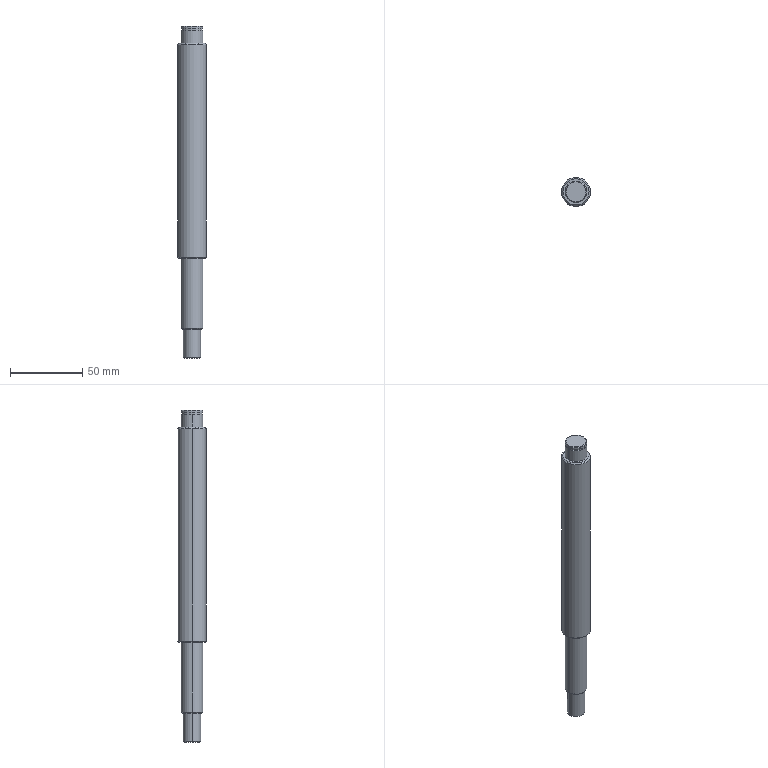Part | SolidWorks | features BaseBody 1 | 1 solid | 29 faces | box 20 x 20 x 230 mm | volume 59762 mm3 | cylinder 12 | cone 10 | plane 7 | commonest cylinder face diameters 15 x6 12 x2 14.3 x2 20 x2
STEP:
#1=CARTESIAN_POINT('',(-5.5,0.,-230.));
#2=VERTEX_POINT('',#1);
#3=CARTESIAN_POINT('',(5.5,0.,-230.));
#4=VERTEX_POINT('',#3);
#5=CARTESIAN_POINT('',(0.,0.,-230.));
#6=DIRECTION('',(0.,0.,-1.));
#7=DIRECTION('',(-1.,0.,0.));
#8=AXIS2_PLACEMENT_3D('',#5,#6,#7);
#9=CIRCLE('',#8,5.5);
#10=EDGE_CURVE('',#2,#4,#9,.T.);
#11=ORIENTED_EDGE('',*,*,#10,.F.);
#12=CARTESIAN_POINT('',(-6.,0.,-229.5));
#13=VERTEX_POINT('',#12);
#14=CARTESIAN_POINT('',(-6.,0.,-229.5));
#15=DIRECTION('',(-0.7071,0.,0.7071));
#16=VECTOR('',#15,1000.);
#17=LINE('',#14,#16);
#18=EDGE_CURVE('',#2,#13,#17,.T.);
#19=ORIENTED_EDGE('',*,*,#18,.T.);
#20=CARTESIAN_POINT('',(6.,0.,-229.5));
#21=VERTEX_POINT('',#20);
#22=CARTESIAN_POINT('',(0.,0.,-229.5));
#23=DIRECTION('',(0.,0.,-1.));
#24=DIRECTION('',(-1.,0.,0.));
#25=AXIS2_PLACEMENT_3D('',#22,#23,#24);
#26=CIRCLE('',#25,6.);
#27=EDGE_CURVE('',#13,#21,#26,.T.);
#28=ORIENTED_EDGE('',*,*,#27,.T.);
#29=CARTESIAN_POINT('',(6.,0.,-229.5));
#30=DIRECTION('',(0.7071,0.,0.7071));
#31=VECTOR('',#30,1000.);
#32=LINE('',#29,#31);
#33=EDGE_CURVE('',#4,#21,#32,.T.);
#34=ORIENTED_EDGE('',*,*,#33,.F.);
#35=EDGE_LOOP('',(#11,#19,#28,#34));
#36=FACE_OUTER_BOUND('',#35,.T.);
#37=CARTESIAN_POINT('',(0.,0.,-229.5));
#38=DIRECTION('',(0.,0.,1.));
#39=DIRECTION('',(1.,0.,0.));
#40=AXIS2_PLACEMENT_3D('',#37,#38,#39);
#41=CONICAL_SURFACE('',#40,6.,0.7854);
#42=ADVANCED_FACE('',(#36),#41,.T.);
#43=CARTESIAN_POINT('',(-6.,0.,-210.));
#44=VERTEX_POINT('',#43);
#45=CARTESIAN_POINT('',(6.,0.,-210.));
#46=VERTEX_POINT('',#45);
#47=CARTESIAN_POINT('',(0.,0.,-210.));
#48=DIRECTION('',(0.,0.,-1.));
#49=DIRECTION('',(-1.,0.,0.));
#50=AXIS2_PLACEMENT_3D('',#47,#48,#49);
#51=CIRCLE('',#50,6.);
#52=EDGE_CURVE('',#44,#46,#51,.T.);
#53=ORIENTED_EDGE('',*,*,#52,.T.);
#54=CARTESIAN_POINT('',(6.,0.,-230.));
#55=DIRECTION('',(0.,0.,-1.));
#56=VECTOR('',#55,1000.);
#57=LINE('',#54,#56);
#58=EDGE_CURVE('',#46,#21,#57,.T.);
#59=ORIENTED_EDGE('',*,*,#58,.T.);
#60=ORIENTED_EDGE('',*,*,#27,.F.);
#61=CARTESIAN_POINT('',(-6.,0.,-230.));
#62=DIRECTION('',(0.,0.,-1.));
#63=VECTOR('',#62,1000.);
#64=LINE('',#61,#63);
#65=EDGE_CURVE('',#44,#13,#64,.T.);
#66=ORIENTED_EDGE('',*,*,#65,.F.);
#67=EDGE_LOOP('',(#53,#59,#60,#66));
#68=FACE_OUTER_BOUND('',#67,.T.);
#69=CARTESIAN_POINT('',(0.,0.,-230.));
#70=DIRECTION('',(0.,0.,-1.));
#71=DIRECTION('',(-1.,0.,0.));
#72=AXIS2_PLACEMENT_3D('',#69,#70,#71);
#73=CYLINDRICAL_SURFACE('',#72,6.);
#74=ADVANCED_FACE('',(#68),#73,.T.);
#75=CARTESIAN_POINT('',(-6.886,0.,-210.));
#76=VERTEX_POINT('',#75);
#77=CARTESIAN_POINT('',(6.886,0.,-210.));
#78=VERTEX_POINT('',#77);
#79=CARTESIAN_POINT('',(0.,0.,-210.));
#80=DIRECTION('',(0.,0.,-1.));
#81=DIRECTION('',(-1.,0.,0.));
#82=AXIS2_PLACEMENT_3D('',#79,#80,#81);
#83=CIRCLE('',#82,6.886);
#84=EDGE_CURVE('',#76,#78,#83,.T.);
#85=ORIENTED_EDGE('',*,*,#84,.F.);
#86=CARTESIAN_POINT('',(-7.5,0.,-209.387));
#87=VERTEX_POINT('',#86);
#88=CARTESIAN_POINT('',(-7.5,0.,-209.387));
#89=DIRECTION('',(-0.7071,0.,0.7071));
#90=VECTOR('',#89,1000.);
#91=LINE('',#88,#90);
#92=EDGE_CURVE('',#76,#87,#91,.T.);
#93=ORIENTED_EDGE('',*,*,#92,.T.);
#94=CARTESIAN_POINT('',(7.5,0.,-209.387));
#95=VERTEX_POINT('',#94);
#96=CARTESIAN_POINT('',(0.,0.,-209.387));
#97=DIRECTION('',(0.,0.,-1.));
#98=DIRECTION('',(-1.,0.,0.));
#99=AXIS2_PLACEMENT_3D('',#96,#97,#98);
#100=CIRCLE('',#99,7.5);
#101=EDGE_CURVE('',#87,#95,#100,.T.);
#102=ORIENTED_EDGE('',*,*,#101,.T.);
#103=CARTESIAN_POINT('',(7.5,0.,-209.387));
#104=DIRECTION('',(0.7071,0.,0.7071));
#105=VECTOR('',#104,1000.);
#106=LINE('',#103,#105);
#107=EDGE_CURVE('',#78,#95,#106,.T.);
#108=ORIENTED_EDGE('',*,*,#107,.F.);
#109=EDGE_LOOP('',(#85,#93,#102,#108));
#110=FACE_OUTER_BOUND('',#109,.T.);
#111=CARTESIAN_POINT('',(0.,0.,-209.387));
#112=DIRECTION('',(0.,0.,1.));
#113=DIRECTION('',(1.,0.,0.));
#114=AXIS2_PLACEMENT_3D('',#111,#112,#113);
#115=CONICAL_SURFACE('',#114,7.5,0.7854);
#116=ADVANCED_FACE('',(#110),#115,.T.);
#117=CARTESIAN_POINT('',(-7.5,0.,-161.));
#118=VERTEX_POINT('',#117);
#119=CARTESIAN_POINT('',(7.5,0.,-161.));
#120=VERTEX_POINT('',#119);
#121=CARTESIAN_POINT('',(0.,0.,-161.));
#122=DIRECTION('',(0.,0.,-1.));
#123=DIRECTION('',(-1.,0.,0.));
#124=AXIS2_PLACEMENT_3D('',#121,#122,#123);
#125=CIRCLE('',#124,7.5);
#126=EDGE_CURVE('',#118,#120,#125,.T.);
#127=ORIENTED_EDGE('',*,*,#126,.T.);
#128=CARTESIAN_POINT('',(7.5,0.,-230.));
#129=DIRECTION('',(0.,0.,-1.));
#130=VECTOR('',#129,1000.);
#131=LINE('',#128,#130);
#132=EDGE_CURVE('',#120,#95,#131,.T.);
#133=ORIENTED_EDGE('',*,*,#132,.T.);
#134=ORIENTED_EDGE('',*,*,#101,.F.);
#135=CARTESIAN_POINT('',(-7.5,0.,-230.));
#136=DIRECTION('',(0.,0.,-1.));
#137=VECTOR('',#136,1000.);
#138=LINE('',#135,#137);
#139=EDGE_CURVE('',#118,#87,#138,.T.);
#140=ORIENTED_EDGE('',*,*,#139,.F.);
#141=EDGE_LOOP('',(#127,#133,#134,#140));
#142=FACE_OUTER_BOUND('',#141,.T.);
#143=CARTESIAN_POINT('',(0.,0.,-230.));
#144=DIRECTION('',(0.,0.,-1.));
#145=DIRECTION('',(-1.,0.,0.));
#146=AXIS2_PLACEMENT_3D('',#143,#144,#145);
#147=CYLINDRICAL_SURFACE('',#146,7.5);
#148=ADVANCED_FACE('',(#142),#147,.T.);
#149=CARTESIAN_POINT('',(-9.08,0.,-161.));
#150=VERTEX_POINT('',#149);
#151=CARTESIAN_POINT('',(9.08,0.,-161.));
#152=VERTEX_POINT('',#151);
#153=CARTESIAN_POINT('',(0.,0.,-161.));
#154=DIRECTION('',(0.,0.,-1.));
#155=DIRECTION('',(-1.,0.,0.));
#156=AXIS2_PLACEMENT_3D('',#153,#154,#155);
#157=CIRCLE('',#156,9.08);
#158=EDGE_CURVE('',#150,#152,#157,.T.);
#159=ORIENTED_EDGE('',*,*,#158,.F.);
#160=CARTESIAN_POINT('',(-10.,0.,-160.08));
#161=VERTEX_POINT('',#160);
#162=CARTESIAN_POINT('',(-10.,0.,-160.08));
#163=DIRECTION('',(-0.7071,0.,0.7071));
#164=VECTOR('',#163,1000.);
#165=LINE('',#162,#164);
#166=EDGE_CURVE('',#150,#161,#165,.T.);
#167=ORIENTED_EDGE('',*,*,#166,.T.);
#168=CARTESIAN_POINT('',(10.,0.,-160.08));
#169=VERTEX_POINT('',#168);
#170=CARTESIAN_POINT('',(0.,0.,-160.08));
#171=DIRECTION('',(0.,0.,-1.));
#172=DIRECTION('',(-1.,0.,0.));
#173=AXIS2_PLACEMENT_3D('',#170,#171,#172);
#174=CIRCLE('',#173,10.);
#175=EDGE_CURVE('',#161,#169,#174,.T.);
#176=ORIENTED_EDGE('',*,*,#175,.T.);
#177=CARTESIAN_POINT('',(10.,0.,-160.08));
#178=DIRECTION('',(0.7071,0.,0.7071));
#179=VECTOR('',#178,1000.);
#180=LINE('',#177,#179);
#181=EDGE_CURVE('',#152,#169,#180,.T.);
#182=ORIENTED_EDGE('',*,*,#181,.F.);
#183=EDGE_LOOP('',(#159,#167,#176,#182));
#184=FACE_OUTER_BOUND('',#183,.T.);
#185=CARTESIAN_POINT('',(0.,0.,-160.08));
#186=DIRECTION('',(0.,0.,1.));
#187=DIRECTION('',(1.,0.,0.));
#188=AXIS2_PLACEMENT_3D('',#185,#186,#187);
#189=CONICAL_SURFACE('',#188,10.,0.7854);
#190=ADVANCED_FACE('',(#184),#189,.T.);
#191=CARTESIAN_POINT('',(-10.,0.,-12.92));
#192=VERTEX_POINT('',#191);
#193=CARTESIAN_POINT('',(10.,0.,-12.92));
#194=VERTEX_POINT('',#193);
#195=CARTESIAN_POINT('',(0.,0.,-12.92));
#196=DIRECTION('',(0.,0.,-1.));
#197=DIRECTION('',(-1.,0.,0.));
#198=AXIS2_PLACEMENT_3D('',#195,#196,#197);
#199=CIRCLE('',#198,10.);
#200=EDGE_CURVE('',#192,#194,#199,.T.);
#201=ORIENTED_EDGE('',*,*,#200,.T.);
#202=CARTESIAN_POINT('',(10.,0.,-230.));
#203=DIRECTION('',(0.,0.,-1.));
#204=VECTOR('',#203,1000.);
#205=LINE('',#202,#204);
#206=EDGE_CURVE('',#194,#169,#205,.T.);
#207=ORIENTED_EDGE('',*,*,#206,.T.);
#208=ORIENTED_EDGE('',*,*,#175,.F.);
#209=CARTESIAN_POINT('',(-10.,0.,-230.));
#210=DIRECTION('',(0.,0.,-1.));
#211=VECTOR('',#210,1000.);
#212=LINE('',#209,#211);
#213=EDGE_CURVE('',#192,#161,#212,.T.);
#214=ORIENTED_EDGE('',*,*,#213,.F.);
#215=EDGE_LOOP('',(#201,#207,#208,#214));
#216=FACE_OUTER_BOUND('',#215,.T.);
#217=CARTESIAN_POINT('',(0.,0.,-230.));
#218=DIRECTION('',(0.,0.,-1.));
#219=DIRECTION('',(-1.,0.,0.));
#220=AXIS2_PLACEMENT_3D('',#217,#218,#219);
#221=CYLINDRICAL_SURFACE('',#220,10.);
#222=ADVANCED_FACE('',(#216),#221,.T.);
#223=CARTESIAN_POINT('',(-9.08,0.,-12.));
#224=VERTEX_POINT('',#223);
#225=CARTESIAN_POINT('',(9.08,0.,-12.));
#226=VERTEX_POINT('',#225);
#227=CARTESIAN_POINT('',(0.,0.,-12.));
#228=DIRECTION('',(0.,0.,-1.));
#229=DIRECTION('',(-1.,0.,0.));
#230=AXIS2_PLACEMENT_3D('',#227,#228,#229);
#231=CIRCLE('',#230,9.08);
#232=EDGE_CURVE('',#224,#226,#231,.T.);
#233=ORIENTED_EDGE('',*,*,#232,.T.);
#234=CARTESIAN_POINT('',(9.08,0.,-12.));
#235=DIRECTION('',(0.7071,0.,-0.7071));
#236=VECTOR('',#235,1000.);
#237=LINE('',#234,#236);
#238=EDGE_CURVE('',#226,#194,#237,.T.);
#239=ORIENTED_EDGE('',*,*,#238,.T.);
#240=ORIENTED_EDGE('',*,*,#200,.F.);
#241=CARTESIAN_POINT('',(-9.08,0.,-12.));
#242=DIRECTION('',(-0.7071,0.,-0.7071));
#243=VECTOR('',#242,1000.);
#244=LINE('',#241,#243);
#245=EDGE_CURVE('',#224,#192,#244,.T.);
#246=ORIENTED_EDGE('',*,*,#245,.F.);
#247=EDGE_LOOP('',(#233,#239,#240,#246));
#248=FACE_OUTER_BOUND('',#247,.T.);
#249=CARTESIAN_POINT('',(0.,0.,-12.));
#250=DIRECTION('',(0.,0.,-1.));
#251=DIRECTION('',(-1.,0.,0.));
#252=AXIS2_PLACEMENT_3D('',#249,#250,#251);
#253=CONICAL_SURFACE('',#252,9.08,0.7854);
#254=ADVANCED_FACE('',(#248),#253,.T.);
#255=CARTESIAN_POINT('',(-7.5,0.,-3.));
#256=VERTEX_POINT('',#255);
#257=CARTESIAN_POINT('',(7.5,0.,-3.));
#258=VERTEX_POINT('',#257);
#259=CARTESIAN_POINT('',(0.,0.,-3.));
#260=DIRECTION('',(0.,0.,-1.));
#261=DIRECTION('',(-1.,0.,0.));
#262=AXIS2_PLACEMENT_3D('',#259,#260,#261);
#263=CIRCLE('',#262,7.5);
#264=EDGE_CURVE('',#256,#258,#263,.T.);
#265=ORIENTED_EDGE('',*,*,#264,.T.);
#266=CARTESIAN_POINT('',(7.5,0.,-12.));
#267=VERTEX_POINT('',#266);
#268=CARTESIAN_POINT('',(7.5,0.,-230.));
#269=DIRECTION('',(0.,0.,-1.));
#270=VECTOR('',#269,1000.);
#271=LINE('',#268,#270);
#272=EDGE_CURVE('',#258,#267,#271,.T.);
#273=ORIENTED_EDGE('',*,*,#272,.T.);
#274=CARTESIAN_POINT('',(-7.5,0.,-12.));
#275=VERTEX_POINT('',#274);
#276=CARTESIAN_POINT('',(0.,0.,-12.));
#277=DIRECTION('',(0.,0.,-1.));
#278=DIRECTION('',(-1.,0.,0.));
#279=AXIS2_PLACEMENT_3D('',#276,#277,#278);
#280=CIRCLE('',#279,7.5);
#281=EDGE_CURVE('',#275,#267,#280,.T.);
#282=ORIENTED_EDGE('',*,*,#281,.F.);
#283=CARTESIAN_POINT('',(-7.5,0.,-230.));
#284=DIRECTION('',(0.,0.,-1.));
#285=VECTOR('',#284,1000.);
#286=LINE('',#283,#285);
#287=EDGE_CURVE('',#256,#275,#286,.T.);
#288=ORIENTED_EDGE('',*,*,#287,.F.);
#289=EDGE_LOOP('',(#265,#273,#282,#288));
#290=FACE_OUTER_BOUND('',#289,.T.);
#291=CARTESIAN_POINT('',(0.,0.,-230.));
#292=DIRECTION('',(0.,0.,-1.));
#293=DIRECTION('',(-1.,0.,0.));
#294=AXIS2_PLACEMENT_3D('',#291,#292,#293);
#295=CYLINDRICAL_SURFACE('',#294,7.5);
#296=ADVANCED_FACE('',(#290),#295,.T.);
#297=CARTESIAN_POINT('',(-7.15,0.,-1.85));
#298=VERTEX_POINT('',#297);
#299=CARTESIAN_POINT('',(7.15,0.,-1.85));
#300=VERTEX_POINT('',#299);
#301=CARTESIAN_POINT('',(0.,0.,-1.85));
#302=DIRECTION('',(0.,0.,-1.));
#303=DIRECTION('',(-1.,0.,0.));
#304=AXIS2_PLACEMENT_3D('',#301,#302,#303);
#305=CIRCLE('',#304,7.15);
#306=EDGE_CURVE('',#298,#300,#305,.T.);
#307=ORIENTED_EDGE('',*,*,#306,.T.);
#308=CARTESIAN_POINT('',(7.15,0.,-3.));
#309=VERTEX_POINT('',#308);
#310=CARTESIAN_POINT('',(7.15,0.,-230.));
#311=DIRECTION('',(0.,0.,-1.));
#312=VECTOR('',#311,1000.);
#313=LINE('',#310,#312);
#314=EDGE_CURVE('',#300,#309,#313,.T.);
#315=ORIENTED_EDGE('',*,*,#314,.T.);
#316=CARTESIAN_POINT('',(-7.15,0.,-3.));
#317=VERTEX_POINT('',#316);
#318=CARTESIAN_POINT('',(0.,0.,-3.));
#319=DIRECTION('',(0.,0.,-1.));
#320=DIRECTION('',(-1.,0.,0.));
#321=AXIS2_PLACEMENT_3D('',#318,#319,#320);
#322=CIRCLE('',#321,7.15);
#323=EDGE_CURVE('',#317,#309,#322,.T.);
#324=ORIENTED_EDGE('',*,*,#323,.F.);
#325=CARTESIAN_POINT('',(-7.15,0.,-230.));
#326=DIRECTION('',(0.,0.,-1.));
#327=VECTOR('',#326,1000.);
#328=LINE('',#325,#327);
#329=EDGE_CURVE('',#298,#317,#328,.T.);
#330=ORIENTED_EDGE('',*,*,#329,.F.);
#331=EDGE_LOOP('',(#307,#315,#324,#330));
#332=FACE_OUTER_BOUND('',#331,.T.);
#333=CARTESIAN_POINT('',(0.,0.,-230.));
#334=DIRECTION('',(0.,0.,-1.));
#335=DIRECTION('',(-1.,0.,0.));
#336=AXIS2_PLACEMENT_3D('',#333,#334,#335);
#337=CYLINDRICAL_SURFACE('',#336,7.15);
#338=ADVANCED_FACE('',(#332),#337,.T.);
#339=CARTESIAN_POINT('',(-7.5,0.,-0.5));
#340=VERTEX_POINT('',#339);
#341=CARTESIAN_POINT('',(7.5,0.,-0.5));
#342=VERTEX_POINT('',#341);
#343=CARTESIAN_POINT('',(0.,0.,-0.5));
#344=DIRECTION('',(0.,0.,-1.));
#345=DIRECTION('',(-1.,0.,0.));
#346=AXIS2_PLACEMENT_3D('',#343,#344,#345);
#347=CIRCLE('',#346,7.5);
#348=EDGE_CURVE('',#340,#342,#347,.T.);
#349=ORIENTED_EDGE('',*,*,#348,.T.);
#350=CARTESIAN_POINT('',(7.5,0.,-1.85));
#351=VERTEX_POINT('',#350);
#352=CARTESIAN_POINT('',(7.5,0.,-230.));
#353=DIRECTION('',(0.,0.,-1.));
#354=VECTOR('',#353,1000.);
#355=LINE('',#352,#354);
#356=EDGE_CURVE('',#342,#351,#355,.T.);
#357=ORIENTED_EDGE('',*,*,#356,.T.);
#358=CARTESIAN_POINT('',(-7.5,0.,-1.85));
#359=VERTEX_POINT('',#358);
#360=CARTESIAN_POINT('',(0.,0.,-1.85));
#361=DIRECTION('',(0.,0.,-1.));
#362=DIRECTION('',(-1.,0.,0.));
#363=AXIS2_PLACEMENT_3D('',#360,#361,#362);
#364=CIRCLE('',#363,7.5);
#365=EDGE_CURVE('',#359,#351,#364,.T.);
#366=ORIENTED_EDGE('',*,*,#365,.F.);
#367=CARTESIAN_POINT('',(-7.5,0.,-230.));
#368=DIRECTION('',(0.,0.,-1.));
#369=VECTOR('',#368,1000.);
#370=LINE('',#367,#369);
#371=EDGE_CURVE('',#340,#359,#370,.T.);
#372=ORIENTED_EDGE('',*,*,#371,.F.);
#373=EDGE_LOOP('',(#349,#357,#366,#372));
#374=FACE_OUTER_BOUND('',#373,.T.);
#375=CARTESIAN_POINT('',(0.,0.,-230.));
#376=DIRECTION('',(0.,0.,-1.));
#377=DIRECTION('',(-1.,0.,0.));
#378=AXIS2_PLACEMENT_3D('',#375,#376,#377);
#379=CYLINDRICAL_SURFACE('',#378,7.5);
#380=ADVANCED_FACE('',(#374),#379,.T.);
#381=CARTESIAN_POINT('',(-7.,0.,0.));
#382=VERTEX_POINT('',#381);
#383=CARTESIAN_POINT('',(7.,0.,0.));
#384=VERTEX_POINT('',#383);
#385=CARTESIAN_POINT('',(0.,0.,0.));
#386=DIRECTION('',(0.,0.,-1.));
#387=DIRECTION('',(-1.,0.,0.));
#388=AXIS2_PLACEMENT_3D('',#385,#386,#387);
#389=CIRCLE('',#388,7.);
#390=EDGE_CURVE('',#382,#384,#389,.T.);
#391=ORIENTED_EDGE('',*,*,#390,.T.);
#392=CARTESIAN_POINT('',(7.,0.,0.));
#393=DIRECTION('',(0.7071,0.,-0.7071));
#394=VECTOR('',#393,1000.);
#395=LINE('',#392,#394);
#396=EDGE_CURVE('',#384,#342,#395,.T.);
#397=ORIENTED_EDGE('',*,*,#396,.T.);
#398=ORIENTED_EDGE('',*,*,#348,.F.);
#399=CARTESIAN_POINT('',(-7.,0.,0.));
#400=DIRECTION('',(-0.7071,0.,-0.7071));
#401=VECTOR('',#400,1000.);
#402=LINE('',#399,#401);
#403=EDGE_CURVE('',#382,#340,#402,.T.);
#404=ORIENTED_EDGE('',*,*,#403,.F.);
#405=EDGE_LOOP('',(#391,#397,#398,#404));
#406=FACE_OUTER_BOUND('',#405,.T.);
#407=CARTESIAN_POINT('',(0.,0.,0.));
#408=DIRECTION('',(0.,0.,-1.));
#409=DIRECTION('',(-1.,0.,0.));
#410=AXIS2_PLACEMENT_3D('',#407,#408,#409);
#411=CONICAL_SURFACE('',#410,7.,0.7854);
#412=ADVANCED_FACE('',(#406),#411,.T.);
#413=CARTESIAN_POINT('',(0.,0.,-230.));
#414=DIRECTION('',(0.,0.,-1.));
#415=DIRECTION('',(-1.,0.,0.));
#416=AXIS2_PLACEMENT_3D('',#413,#414,#415);
#417=CIRCLE('',#416,5.5);
#418=EDGE_CURVE('',#4,#2,#417,.T.);
#419=ORIENTED_EDGE('',*,*,#418,.T.);
#420=ORIENTED_EDGE('',*,*,#10,.T.);
#421=EDGE_LOOP('',(#419,#420));
#422=FACE_OUTER_BOUND('',#421,.T.);
#423=CARTESIAN_POINT('',(0.,5.5,-230.));
#424=DIRECTION('',(0.,0.,1.));
#425=DIRECTION('',(1.,0.,0.));
#426=AXIS2_PLACEMENT_3D('',#423,#424,#425);
#427=PLANE('',#426);
#428=ADVANCED_FACE('',(#422),#427,.F.);
#429=ORIENTED_EDGE('',*,*,#52,.F.);
#430=CARTESIAN_POINT('',(0.,0.,-210.));
#431=DIRECTION('',(0.,0.,-1.));
#432=DIRECTION('',(-1.,0.,0.));
#433=AXIS2_PLACEMENT_3D('',#430,#431,#432);
#434=CIRCLE('',#433,6.);
#435=EDGE_CURVE('',#46,#44,#434,.T.);
#436=ORIENTED_EDGE('',*,*,#435,.F.);
#437=EDGE_LOOP('',(#429,#436));
#438=FACE_BOUND('',#437,.T.);
#439=CARTESIAN_POINT('',(0.,0.,-210.));
#440=DIRECTION('',(0.,0.,-1.));
#441=DIRECTION('',(-1.,0.,0.));
#442=AXIS2_PLACEMENT_3D('',#439,#440,#441);
#443=CIRCLE('',#442,6.886);
#444=EDGE_CURVE('',#78,#76,#443,.T.);
#445=ORIENTED_EDGE('',*,*,#444,.T.);
#446=ORIENTED_EDGE('',*,*,#84,.T.);
#447=EDGE_LOOP('',(#445,#446));
#448=FACE_OUTER_BOUND('',#447,.T.);
#449=CARTESIAN_POINT('',(0.,6.886,-210.));
#450=DIRECTION('',(0.,0.,1.));
#451=DIRECTION('',(1.,0.,0.));
#452=AXIS2_PLACEMENT_3D('',#449,#450,#451);
#453=PLANE('',#452);
#454=ADVANCED_FACE('',(#438,#448),#453,.F.);
#455=ORIENTED_EDGE('',*,*,#126,.F.);
#456=CARTESIAN_POINT('',(0.,0.,-161.));
#457=DIRECTION('',(0.,0.,-1.));
#458=DIRECTION('',(-1.,0.,0.));
#459=AXIS2_PLACEMENT_3D('',#456,#457,#458);
#460=CIRCLE('',#459,7.5);
#461=EDGE_CURVE('',#120,#118,#460,.T.);
#462=ORIENTED_EDGE('',*,*,#461,.F.);
#463=EDGE_LOOP('',(#455,#462));
#464=FACE_BOUND('',#463,.T.);
#465=CARTESIAN_POINT('',(0.,0.,-161.));
#466=DIRECTION('',(0.,0.,-1.));
#467=DIRECTION('',(-1.,0.,0.));
#468=AXIS2_PLACEMENT_3D('',#465,#466,#467);
#469=CIRCLE('',#468,9.08);
#470=EDGE_CURVE('',#152,#150,#469,.T.);
#471=ORIENTED_EDGE('',*,*,#470,.T.);
#472=ORIENTED_EDGE('',*,*,#158,.T.);
#473=EDGE_LOOP('',(#471,#472));
#474=FACE_OUTER_BOUND('',#473,.T.);
#475=CARTESIAN_POINT('',(0.,9.08,-161.));
#476=DIRECTION('',(0.,0.,1.));
#477=DIRECTION('',(1.,0.,0.));
#478=AXIS2_PLACEMENT_3D('',#475,#476,#477);
#479=PLANE('',#478);
#480=ADVANCED_FACE('',(#464,#474),#479,.F.);
#481=ORIENTED_EDGE('',*,*,#281,.T.);
#482=CARTESIAN_POINT('',(0.,0.,-12.));
#483=DIRECTION('',(0.,0.,-1.));
#484=DIRECTION('',(-1.,0.,0.));
#485=AXIS2_PLACEMENT_3D('',#482,#483,#484);
#486=CIRCLE('',#485,7.5);
#487=EDGE_CURVE('',#267,#275,#486,.T.);
#488=ORIENTED_EDGE('',*,*,#487,.T.);
#489=EDGE_LOOP('',(#481,#488));
#490=FACE_BOUND('',#489,.T.);
#491=ORIENTED_EDGE('',*,*,#232,.F.);
#492=CARTESIAN_POINT('',(0.,0.,-12.));
#493=DIRECTION('',(0.,0.,-1.));
#494=DIRECTION('',(-1.,0.,0.));
#495=AXIS2_PLACEMENT_3D('',#492,#493,#494);
#496=CIRCLE('',#495,9.08);
#497=EDGE_CURVE('',#226,#224,#496,.T.);
#498=ORIENTED_EDGE('',*,*,#497,.F.);
#499=EDGE_LOOP('',(#491,#498));
#500=FACE_OUTER_BOUND('',#499,.T.);
#501=CARTESIAN_POINT('',(0.,7.5,-12.));
#502=DIRECTION('',(0.,0.,-1.));
#503=DIRECTION('',(0.,-1.,0.));
#504=AXIS2_PLACEMENT_3D('',#501,#502,#503);
#505=PLANE('',#504);
#506=ADVANCED_FACE('',(#490,#500),#505,.F.);
#507=ORIENTED_EDGE('',*,*,#323,.T.);
#508=CARTESIAN_POINT('',(0.,0.,-3.));
#509=DIRECTION('',(0.,0.,-1.));
#510=DIRECTION('',(-1.,0.,0.));
#511=AXIS2_PLACEMENT_3D('',#508,#509,#510);
#512=CIRCLE('',#511,7.15);
#513=EDGE_CURVE('',#309,#317,#512,.T.);
#514=ORIENTED_EDGE('',*,*,#513,.T.);
#515=EDGE_LOOP('',(#507,#514));
#516=FACE_BOUND('',#515,.T.);
#517=ORIENTED_EDGE('',*,*,#264,.F.);
#518=CARTESIAN_POINT('',(0.,0.,-3.));
#519=DIRECTION('',(0.,0.,-1.));
#520=DIRECTION('',(-1.,0.,0.));
#521=AXIS2_PLACEMENT_3D('',#518,#519,#520);
#522=CIRCLE('',#521,7.5);
#523=EDGE_CURVE('',#258,#256,#522,.T.);
#524=ORIENTED_EDGE('',*,*,#523,.F.);
#525=EDGE_LOOP('',(#517,#524));
#526=FACE_OUTER_BOUND('',#525,.T.);
#527=CARTESIAN_POINT('',(0.,7.15,-3.));
#528=DIRECTION('',(0.,0.,-1.));
#529=DIRECTION('',(0.,-1.,0.));
#530=AXIS2_PLACEMENT_3D('',#527,#528,#529);
#531=PLANE('',#530);
#532=ADVANCED_FACE('',(#516,#526),#531,.F.);
#533=ORIENTED_EDGE('',*,*,#306,.F.);
#534=CARTESIAN_POINT('',(0.,0.,-1.85));
#535=DIRECTION('',(0.,0.,-1.));
#536=DIRECTION('',(-1.,0.,0.));
#537=AXIS2_PLACEMENT_3D('',#534,#535,#536);
#538=CIRCLE('',#537,7.15);
#539=EDGE_CURVE('',#300,#298,#538,.T.);
#540=ORIENTED_EDGE('',*,*,#539,.F.);
#541=EDGE_LOOP('',(#533,#540));
#542=FACE_BOUND('',#541,.T.);
#543=ORIENTED_EDGE('',*,*,#365,.T.);
#544=CARTESIAN_POINT('',(0.,0.,-1.85));
#545=DIRECTION('',(0.,0.,-1.));
#546=DIRECTION('',(-1.,0.,0.));
#547=AXIS2_PLACEMENT_3D('',#544,#545,#546);
#548=CIRCLE('',#547,7.5);
#549=EDGE_CURVE('',#351,#359,#548,.T.);
#550=ORIENTED_EDGE('',*,*,#549,.T.);
#551=EDGE_LOOP('',(#543,#550));
#552=FACE_OUTER_BOUND('',#551,.T.);
#553=CARTESIAN_POINT('',(0.,7.5,-1.85));
#554=DIRECTION('',(0.,0.,1.));
#555=DIRECTION('',(1.,0.,0.));
#556=AXIS2_PLACEMENT_3D('',#553,#554,#555);
#557=PLANE('',#556);
#558=ADVANCED_FACE('',(#542,#552),#557,.F.);
#559=ORIENTED_EDGE('',*,*,#390,.F.);
#560=CARTESIAN_POINT('',(0.,0.,0.));
#561=DIRECTION('',(0.,0.,-1.));
#562=DIRECTION('',(-1.,0.,0.));
#563=AXIS2_PLACEMENT_3D('',#560,#561,#562);
#564=CIRCLE('',#563,7.);
#565=EDGE_CURVE('',#384,#382,#564,.T.);
#566=ORIENTED_EDGE('',*,*,#565,.F.);
#567=EDGE_LOOP('',(#559,#566));
#568=FACE_OUTER_BOUND('',#567,.T.);
#569=CARTESIAN_POINT('',(0.,0.,0.));
#570=DIRECTION('',(0.,0.,-1.));
#571=DIRECTION('',(0.,-1.,0.));
#572=AXIS2_PLACEMENT_3D('',#569,#570,#571);
#573=PLANE('',#572);
#574=ADVANCED_FACE('',(#568),#573,.F.);
#575=ORIENTED_EDGE('',*,*,#396,.F.);
#576=ORIENTED_EDGE('',*,*,#565,.T.);
#577=ORIENTED_EDGE('',*,*,#403,.T.);
#578=CARTESIAN_POINT('',(0.,0.,-0.5));
#579=DIRECTION('',(0.,0.,-1.));
#580=DIRECTION('',(-1.,0.,0.));
#581=AXIS2_PLACEMENT_3D('',#578,#579,#580);
#582=CIRCLE('',#581,7.5);
#583=EDGE_CURVE('',#342,#340,#582,.T.);
#584=ORIENTED_EDGE('',*,*,#583,.F.);
#585=EDGE_LOOP('',(#575,#576,#577,#584));
#586=FACE_OUTER_BOUND('',#585,.T.);
#587=CARTESIAN_POINT('',(0.,0.,0.));
#588=DIRECTION('',(0.,0.,-1.));
#589=DIRECTION('',(-1.,0.,0.));
#590=AXIS2_PLACEMENT_3D('',#587,#588,#589);
#591=CONICAL_SURFACE('',#590,7.,0.7854);
#592=ADVANCED_FACE('',(#586),#591,.T.);
#593=ORIENTED_EDGE('',*,*,#356,.F.);
#594=ORIENTED_EDGE('',*,*,#583,.T.);
#595=ORIENTED_EDGE('',*,*,#371,.T.);
#596=ORIENTED_EDGE('',*,*,#549,.F.);
#597=EDGE_LOOP('',(#593,#594,#595,#596));
#598=FACE_OUTER_BOUND('',#597,.T.);
#599=CARTESIAN_POINT('',(0.,0.,-230.));
#600=DIRECTION('',(0.,0.,-1.));
#601=DIRECTION('',(-1.,0.,0.));
#602=AXIS2_PLACEMENT_3D('',#599,#600,#601);
#603=CYLINDRICAL_SURFACE('',#602,7.5);
#604=ADVANCED_FACE('',(#598),#603,.T.);
#605=ORIENTED_EDGE('',*,*,#314,.F.);
#606=ORIENTED_EDGE('',*,*,#539,.T.);
#607=ORIENTED_EDGE('',*,*,#329,.T.);
#608=ORIENTED_EDGE('',*,*,#513,.F.);
#609=EDGE_LOOP('',(#605,#606,#607,#608));
#610=FACE_OUTER_BOUND('',#609,.T.);
#611=CARTESIAN_POINT('',(0.,0.,-230.));
#612=DIRECTION('',(0.,0.,-1.));
#613=DIRECTION('',(-1.,0.,0.));
#614=AXIS2_PLACEMENT_3D('',#611,#612,#613);
#615=CYLINDRICAL_SURFACE('',#614,7.15);
#616=ADVANCED_FACE('',(#610),#615,.T.);
#617=ORIENTED_EDGE('',*,*,#272,.F.);
#618=ORIENTED_EDGE('',*,*,#523,.T.);
#619=ORIENTED_EDGE('',*,*,#287,.T.);
#620=ORIENTED_EDGE('',*,*,#487,.F.);
#621=EDGE_LOOP('',(#617,#618,#619,#620));
#622=FACE_OUTER_BOUND('',#621,.T.);
#623=CARTESIAN_POINT('',(0.,0.,-230.));
#624=DIRECTION('',(0.,0.,-1.));
#625=DIRECTION('',(-1.,0.,0.));
#626=AXIS2_PLACEMENT_3D('',#623,#624,#625);
#627=CYLINDRICAL_SURFACE('',#626,7.5);
#628=ADVANCED_FACE('',(#622),#627,.T.);
#629=ORIENTED_EDGE('',*,*,#238,.F.);
#630=ORIENTED_EDGE('',*,*,#497,.T.);
#631=ORIENTED_EDGE('',*,*,#245,.T.);
#632=CARTESIAN_POINT('',(0.,0.,-12.92));
#633=DIRECTION('',(0.,0.,-1.));
#634=DIRECTION('',(-1.,0.,0.));
#635=AXIS2_PLACEMENT_3D('',#632,#633,#634);
#636=CIRCLE('',#635,10.);
#637=EDGE_CURVE('',#194,#192,#636,.T.);
#638=ORIENTED_EDGE('',*,*,#637,.F.);
#639=EDGE_LOOP('',(#629,#630,#631,#638));
#640=FACE_OUTER_BOUND('',#639,.T.);
#641=CARTESIAN_POINT('',(0.,0.,-12.));
#642=DIRECTION('',(0.,0.,-1.));
#643=DIRECTION('',(-1.,0.,0.));
#644=AXIS2_PLACEMENT_3D('',#641,#642,#643);
#645=CONICAL_SURFACE('',#644,9.08,0.7854);
#646=ADVANCED_FACE('',(#640),#645,.T.);
#647=ORIENTED_EDGE('',*,*,#206,.F.);
#648=ORIENTED_EDGE('',*,*,#637,.T.);
#649=ORIENTED_EDGE('',*,*,#213,.T.);
#650=CARTESIAN_POINT('',(0.,0.,-160.08));
#651=DIRECTION('',(0.,0.,-1.));
#652=DIRECTION('',(-1.,0.,0.));
#653=AXIS2_PLACEMENT_3D('',#650,#651,#652);
#654=CIRCLE('',#653,10.);
#655=EDGE_CURVE('',#169,#161,#654,.T.);
#656=ORIENTED_EDGE('',*,*,#655,.F.);
#657=EDGE_LOOP('',(#647,#648,#649,#656));
#658=FACE_OUTER_BOUND('',#657,.T.);
#659=CARTESIAN_POINT('',(0.,0.,-230.));
#660=DIRECTION('',(0.,0.,-1.));
#661=DIRECTION('',(-1.,0.,0.));
#662=AXIS2_PLACEMENT_3D('',#659,#660,#661);
#663=CYLINDRICAL_SURFACE('',#662,10.);
#664=ADVANCED_FACE('',(#658),#663,.T.);
#665=ORIENTED_EDGE('',*,*,#166,.F.);
#666=ORIENTED_EDGE('',*,*,#470,.F.);
#667=ORIENTED_EDGE('',*,*,#181,.T.);
#668=ORIENTED_EDGE('',*,*,#655,.T.);
#669=EDGE_LOOP('',(#665,#666,#667,#668));
#670=FACE_OUTER_BOUND('',#669,.T.);
#671=CARTESIAN_POINT('',(0.,0.,-160.08));
#672=DIRECTION('',(0.,0.,1.));
#673=DIRECTION('',(1.,0.,0.));
#674=AXIS2_PLACEMENT_3D('',#671,#672,#673);
#675=CONICAL_SURFACE('',#674,10.,0.7854);
#676=ADVANCED_FACE('',(#670),#675,.T.);
#677=ORIENTED_EDGE('',*,*,#132,.F.);
#678=ORIENTED_EDGE('',*,*,#461,.T.);
#679=ORIENTED_EDGE('',*,*,#139,.T.);
#680=CARTESIAN_POINT('',(0.,0.,-209.387));
#681=DIRECTION('',(0.,0.,-1.));
#682=DIRECTION('',(-1.,0.,0.));
#683=AXIS2_PLACEMENT_3D('',#680,#681,#682);
#684=CIRCLE('',#683,7.5);
#685=EDGE_CURVE('',#95,#87,#684,.T.);
#686=ORIENTED_EDGE('',*,*,#685,.F.);
#687=EDGE_LOOP('',(#677,#678,#679,#686));
#688=FACE_OUTER_BOUND('',#687,.T.);
#689=CARTESIAN_POINT('',(0.,0.,-230.));
#690=DIRECTION('',(0.,0.,-1.));
#691=DIRECTION('',(-1.,0.,0.));
#692=AXIS2_PLACEMENT_3D('',#689,#690,#691);
#693=CYLINDRICAL_SURFACE('',#692,7.5);
#694=ADVANCED_FACE('',(#688),#693,.T.);
#695=ORIENTED_EDGE('',*,*,#92,.F.);
#696=ORIENTED_EDGE('',*,*,#444,.F.);
#697=ORIENTED_EDGE('',*,*,#107,.T.);
#698=ORIENTED_EDGE('',*,*,#685,.T.);
#699=EDGE_LOOP('',(#695,#696,#697,#698));
#700=FACE_OUTER_BOUND('',#699,.T.);
#701=CARTESIAN_POINT('',(0.,0.,-209.387));
#702=DIRECTION('',(0.,0.,1.));
#703=DIRECTION('',(1.,0.,0.));
#704=AXIS2_PLACEMENT_3D('',#701,#702,#703);
#705=CONICAL_SURFACE('',#704,7.5,0.7854);
#706=ADVANCED_FACE('',(#700),#705,.T.);
#707=ORIENTED_EDGE('',*,*,#58,.F.);
#708=ORIENTED_EDGE('',*,*,#435,.T.);
#709=ORIENTED_EDGE('',*,*,#65,.T.);
#710=CARTESIAN_POINT('',(0.,0.,-229.5));
#711=DIRECTION('',(0.,0.,-1.));
#712=DIRECTION('',(-1.,0.,0.));
#713=AXIS2_PLACEMENT_3D('',#710,#711,#712);
#714=CIRCLE('',#713,6.);
#715=EDGE_CURVE('',#21,#13,#714,.T.);
#716=ORIENTED_EDGE('',*,*,#715,.F.);
#717=EDGE_LOOP('',(#707,#708,#709,#716));
#718=FACE_OUTER_BOUND('',#717,.T.);
#719=CARTESIAN_POINT('',(0.,0.,-230.));
#720=DIRECTION('',(0.,0.,-1.));
#721=DIRECTION('',(-1.,0.,0.));
#722=AXIS2_PLACEMENT_3D('',#719,#720,#721);
#723=CYLINDRICAL_SURFACE('',#722,6.);
#724=ADVANCED_FACE('',(#718),#723,.T.);
#725=ORIENTED_EDGE('',*,*,#18,.F.);
#726=ORIENTED_EDGE('',*,*,#418,.F.);
#727=ORIENTED_EDGE('',*,*,#33,.T.);
#728=ORIENTED_EDGE('',*,*,#715,.T.);
#729=EDGE_LOOP('',(#725,#726,#727,#728));
#730=FACE_OUTER_BOUND('',#729,.T.);
#731=CARTESIAN_POINT('',(0.,0.,-229.5));
#732=DIRECTION('',(0.,0.,1.));
#733=DIRECTION('',(1.,0.,0.));
#734=AXIS2_PLACEMENT_3D('',#731,#732,#733);
#735=CONICAL_SURFACE('',#734,6.,0.7854);
#736=ADVANCED_FACE('',(#730),#735,.T.);
#737=CLOSED_SHELL('',(#42,#74,#116,#148,#190,#222,#254,#296,#338,#380,#412,#428,#454,#480,#506,#532,#558,#574,#592,#604,#616,#628,#646,#664,#676,#694,#706,#724,#736));
#738=MANIFOLD_SOLID_BREP('',#737);
#739=CARTESIAN_POINT('',(0.,0.,0.));
#740=DIRECTION('',(0.,0.,1.));
#741=DIRECTION('',(1.,0.,0.));
#742=AXIS2_PLACEMENT_3D('',#739,#740,#741);
#743=(LENGTH_UNIT()NAMED_UNIT(*)SI_UNIT(.MILLI.,.METRE.));
#744=UNCERTAINTY_MEASURE_WITH_UNIT(LENGTH_MEASURE(0.00001),#743,'','');
#745=(NAMED_UNIT(*)PLANE_ANGLE_UNIT()SI_UNIT($,.RADIAN.));
#746=(NAMED_UNIT(*)SI_UNIT($,.STERADIAN.)SOLID_ANGLE_UNIT());
#747=(GEOMETRIC_REPRESENTATION_CONTEXT(3)GLOBAL_UNCERTAINTY_ASSIGNED_CONTEXT((#744))GLOBAL_UNIT_ASSIGNED_CONTEXT((#743,#745,#746))REPRESENTATION_CONTEXT('',''));
#748=ADVANCED_BREP_SHAPE_REPRESENTATION('',(#738,#742),#747);